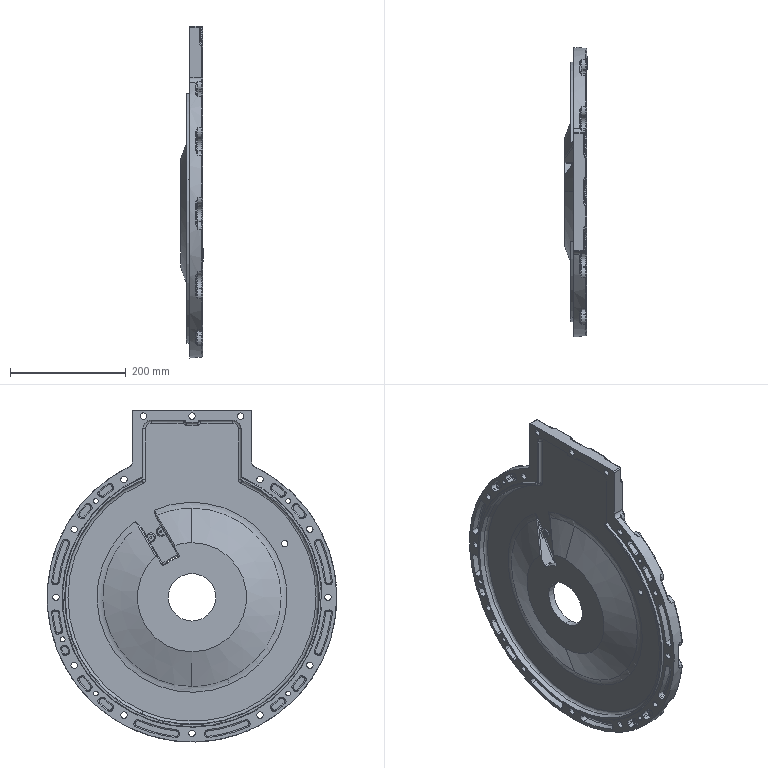Part | SolidWorks | features BaseBody 1 | 1 solid | 1546 faces | box 38.5 x 500 x 573.5 mm | volume 2957583 mm3 | cylinder 613 | torus 489 | plane 194 | spline 162 | cone 76 | sphere 12 | commonest cylinder face diameters 4 x164 20 x74 10 x65 3 x48 22 x37 11 x28